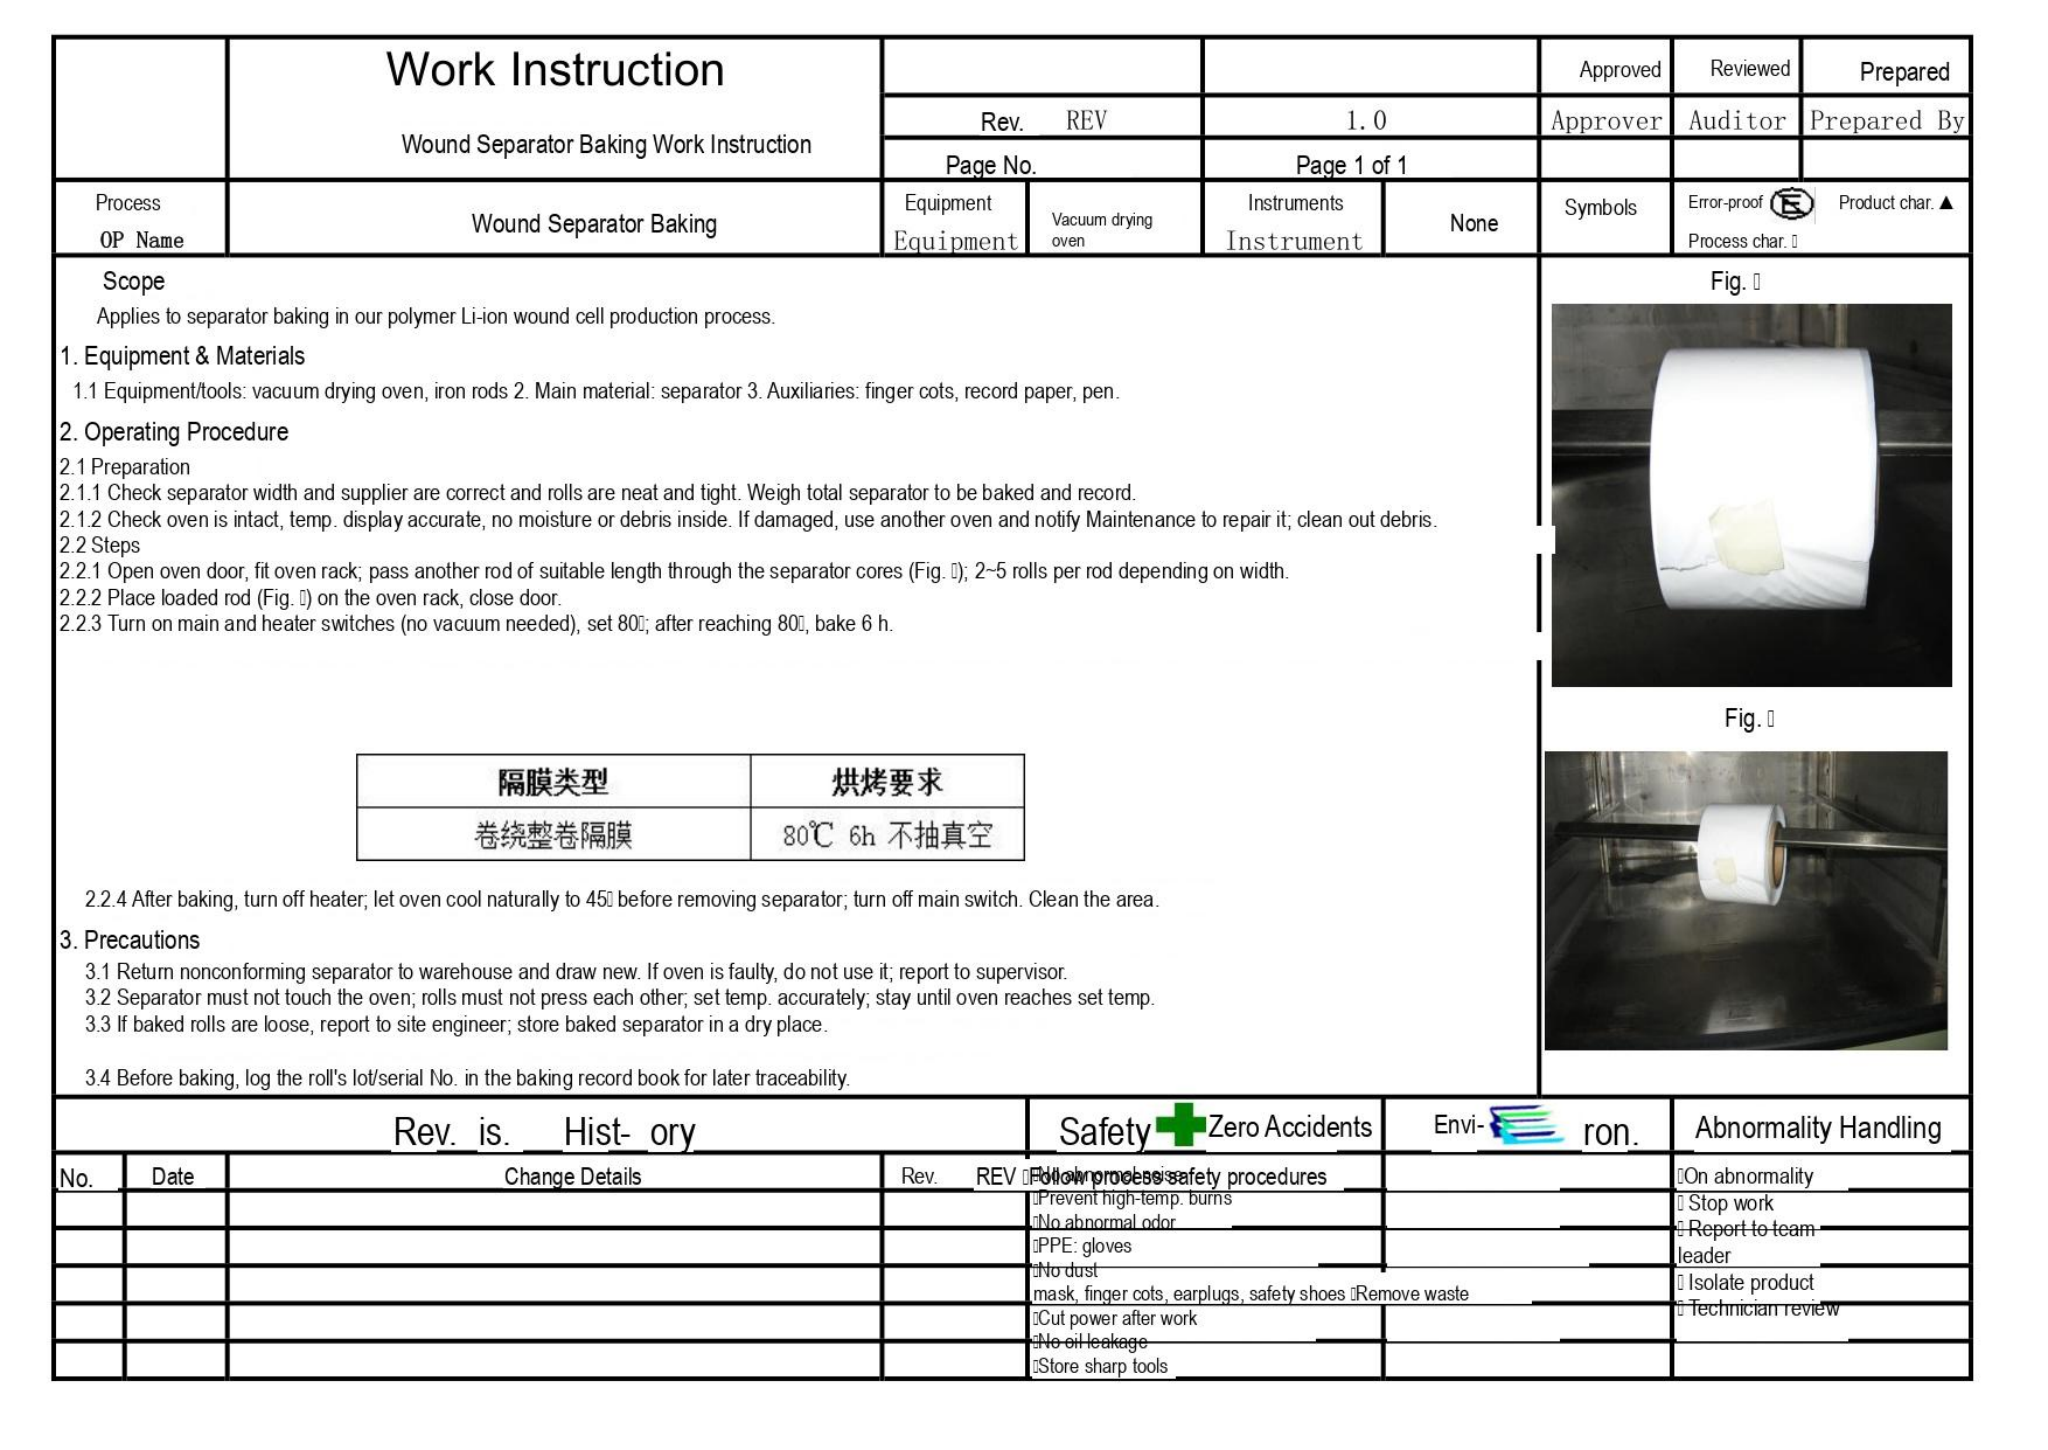# Work Instruction

| | Work Instruction<br>Wound Separator Baking Work Instruction | | | Approved | Reviewed | Prepared |
|---|---|---|---|---|---|---|
| | | Rev. REV | 1.0 | Approver | Auditor | Prepared By |
| | | Page No. | Page 1 of 1 | | | |

| Process<br>OP Name | Wound Separator Baking | Equipment<br>Equipment | Vacuum drying oven | Instruments<br>Instrument | None | Symbols | Error-proof Product char. ▲<br>Process char. |
|---|---|---|---|---|---|---|---|

**Scope**
Applies to separator baking in our polymer Li-ion wound cell production process.

**1. Equipment & Materials**
1.1 Equipment/tools: vacuum drying oven, iron rods 2. Main material: separator 3. Auxiliaries: finger cots, record paper, pen.

**2. Operating Procedure**
2.1 Preparation
2.1.1 Check separator width and supplier are correct and rolls are neat and tight. Weigh total separator to be baked and record.
2.1.2 Check oven is intact, temp. display accurate, no moisture or debris inside. If damaged, use another oven and notify Maintenance to repair it; clean out debris.
2.2 Steps
2.2.1 Open oven door, fit oven rack; pass another rod of suitable length through the separator cores (Fig. ); 2~5 rolls per rod depending on width.
2.2.2 Place loaded rod (Fig. ) on the oven rack, close door.
2.2.3 Turn on main and heater switches (no vacuum needed), set 80; after reaching 80, bake 6 h.

| 隔膜类型 | 烘烤要求 |
|---|---|
| 卷绕整卷隔膜 | 80℃ 6h 不抽真空 |

2.2.4 After baking, turn off heater; let oven cool naturally to 45 before removing separator; turn off main switch. Clean the area.

**3. Precautions**
3.1 Return nonconforming separator to warehouse and draw new. If oven is faulty, do not use it; report to supervisor.
3.2 Separator must not touch the oven; rolls must not press each other; set temp. accurately; stay until oven reaches set temp.
3.3 If baked rolls are loose, report to site engineer; store baked separator in a dry place.

3.4 Before baking, log the roll's lot/serial No. in the baking record book for later traceability.

Fig.

Fig.

| Rev. is. Hist- ory | | | | Safety Zero Accidents | Envi- ron. | Abnormality Handling |
|---|---|---|---|---|---|---|
| No. | Date | Change Details | Rev. REV | No abnormal noise<br>Follow process safety procedures<br>Prevent high-temp. burns<br>No abnormal odor<br>PPE: gloves<br>No dust<br>mask, finger cots, earplugs, safety shoes Remove waste<br>Cut power after work<br>No oil leakage<br>Store sharp tools | | On abnormality<br>Stop work<br>Report to team leader<br>Isolate product<br>Technician review |
| | | | | | | |
| | | | | | | |
| | | | | | | |
| | | | | | | |
| | | | | | | |